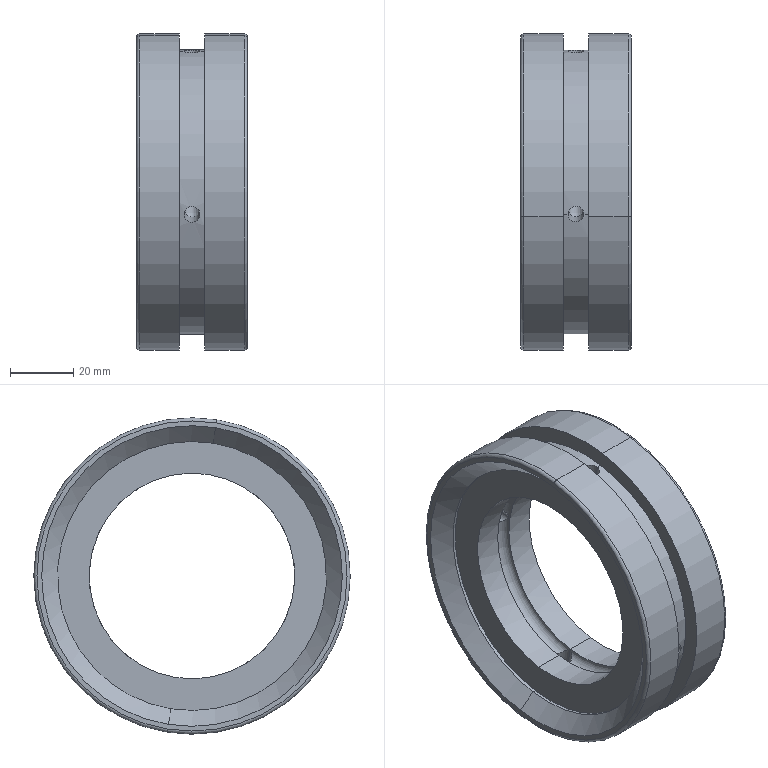Part | STEP file | Input 19 | 1 solid | 40 faces | box 35 x 100 x 100 mm | volume 108578 mm3 | cylinder 22 | torus 8 | plane 6 | cone 4 | commonest cylinder face diameters 5 x8 65 x4 85 x4 100 x4 90 x2